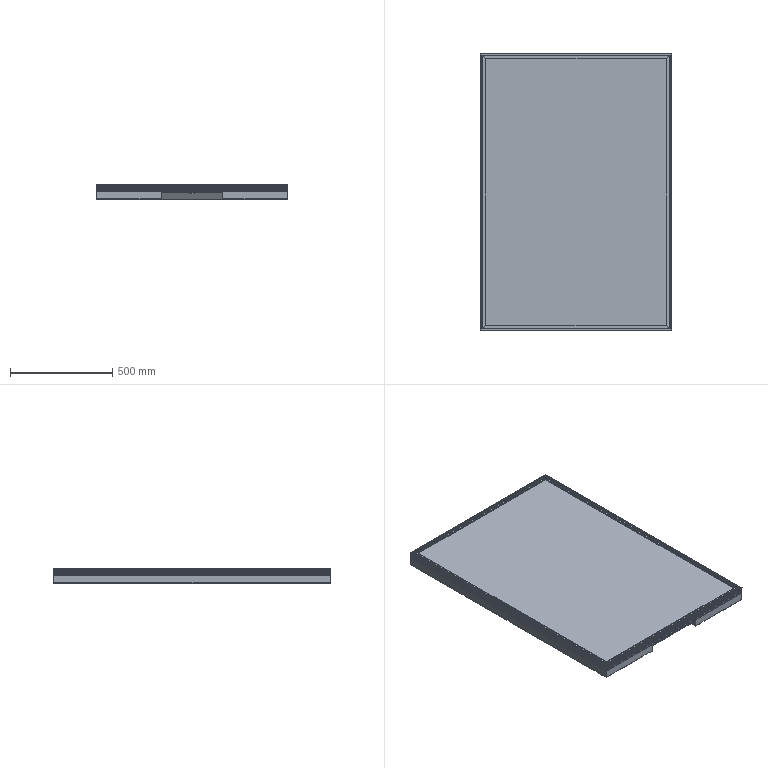Part | SolidWorks | 9 solids | 878 faces | box 940 x 1360 x 70 mm | volume 23825388 mm3 | plane 582 | cylinder 264 | spline 32 | commonest cylinder face diameters 7 x100 0.4 x67 2.4 x41 11 x32 2 x16 1 x8